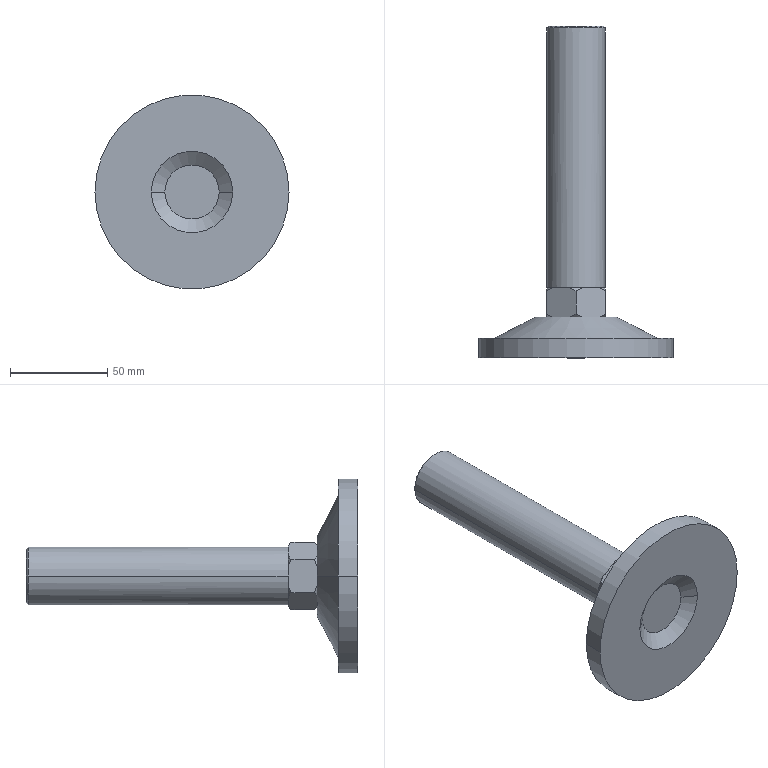Part | SolidWorks | features ICE 3, Chamfer 1, RevCut 1, Revolution 1 | 1 solid | 39 faces | box 100 x 171 x 100 mm | volume 216271 mm3 | cone 18 | plane 17 | cylinder 4 | commonest cylinder face diameters 30 x2 100 x2
STEP:
#1=CARTESIAN_POINT('',(14.,15.,0.));
#2=VERTEX_POINT('',#1);
#3=CARTESIAN_POINT('',(-14.,15.,0.));
#4=VERTEX_POINT('',#3);
#5=CARTESIAN_POINT('',(0.,15.,0.));
#6=DIRECTION('',(0.,1.,0.));
#7=DIRECTION('',(-1.,0.,0.));
#8=AXIS2_PLACEMENT_3D('',#5,#6,#7);
#9=CIRCLE('',#8,14.);
#10=EDGE_CURVE('',#2,#4,#9,.T.);
#11=ORIENTED_EDGE('',*,*,#10,.T.);
#12=CARTESIAN_POINT('',(-21.,10.,0.));
#13=VERTEX_POINT('',#12);
#14=CARTESIAN_POINT('',(-14.,15.,0.));
#15=DIRECTION('',(-0.8137,-0.5812,0.));
#16=VECTOR('',#15,1000.);
#17=LINE('',#14,#16);
#18=EDGE_CURVE('',#4,#13,#17,.T.);
#19=ORIENTED_EDGE('',*,*,#18,.T.);
#20=CARTESIAN_POINT('',(21.,10.,0.));
#21=VERTEX_POINT('',#20);
#22=CARTESIAN_POINT('',(0.,10.,0.));
#23=DIRECTION('',(0.,-1.,0.));
#24=DIRECTION('',(-1.,0.,0.));
#25=AXIS2_PLACEMENT_3D('',#22,#23,#24);
#26=CIRCLE('',#25,21.);
#27=EDGE_CURVE('',#13,#21,#26,.T.);
#28=ORIENTED_EDGE('',*,*,#27,.T.);
#29=CARTESIAN_POINT('',(14.,15.,0.));
#30=DIRECTION('',(0.8137,-0.5812,0.));
#31=VECTOR('',#30,1000.);
#32=LINE('',#29,#31);
#33=EDGE_CURVE('',#2,#21,#32,.T.);
#34=ORIENTED_EDGE('',*,*,#33,.F.);
#35=EDGE_LOOP('',(#11,#19,#28,#34));
#36=FACE_OUTER_BOUND('',#35,.T.);
#37=CARTESIAN_POINT('',(0.,15.,0.));
#38=DIRECTION('',(0.,-1.,0.));
#39=DIRECTION('',(1.,0.,0.));
#40=AXIS2_PLACEMENT_3D('',#37,#38,#39);
#41=CONICAL_SURFACE('',#40,14.,0.9505);
#42=ADVANCED_FACE('',(#36),#41,.F.);
#43=CARTESIAN_POINT('',(50.,10.,0.));
#44=VERTEX_POINT('',#43);
#45=CARTESIAN_POINT('',(-50.,10.,0.));
#46=VERTEX_POINT('',#45);
#47=CARTESIAN_POINT('',(0.,10.,0.));
#48=DIRECTION('',(0.,-1.,0.));
#49=DIRECTION('',(-1.,0.,0.));
#50=AXIS2_PLACEMENT_3D('',#47,#48,#49);
#51=CIRCLE('',#50,50.);
#52=EDGE_CURVE('',#44,#46,#51,.T.);
#53=ORIENTED_EDGE('',*,*,#52,.F.);
#54=CARTESIAN_POINT('',(50.,20.,0.));
#55=VERTEX_POINT('',#54);
#56=CARTESIAN_POINT('',(50.,0.,0.));
#57=DIRECTION('',(0.,1.,0.));
#58=VECTOR('',#57,1000.);
#59=LINE('',#56,#58);
#60=EDGE_CURVE('',#44,#55,#59,.T.);
#61=ORIENTED_EDGE('',*,*,#60,.T.);
#62=CARTESIAN_POINT('',(-50.,20.,0.));
#63=VERTEX_POINT('',#62);
#64=CARTESIAN_POINT('',(0.,20.,0.));
#65=DIRECTION('',(0.,1.,0.));
#66=DIRECTION('',(-1.,0.,0.));
#67=AXIS2_PLACEMENT_3D('',#64,#65,#66);
#68=CIRCLE('',#67,50.);
#69=EDGE_CURVE('',#63,#55,#68,.T.);
#70=ORIENTED_EDGE('',*,*,#69,.F.);
#71=CARTESIAN_POINT('',(-50.,0.,0.));
#72=DIRECTION('',(0.,1.,0.));
#73=VECTOR('',#72,1000.);
#74=LINE('',#71,#73);
#75=EDGE_CURVE('',#46,#63,#74,.T.);
#76=ORIENTED_EDGE('',*,*,#75,.F.);
#77=EDGE_LOOP('',(#53,#61,#70,#76));
#78=FACE_OUTER_BOUND('',#77,.T.);
#79=CARTESIAN_POINT('',(0.,0.,0.));
#80=DIRECTION('',(0.,1.,0.));
#81=DIRECTION('',(-1.,0.,0.));
#82=AXIS2_PLACEMENT_3D('',#79,#80,#81);
#83=CYLINDRICAL_SURFACE('',#82,50.);
#84=ADVANCED_FACE('',(#78),#83,.T.);
#85=CARTESIAN_POINT('',(-14.,181.,0.));
#86=VERTEX_POINT('',#85);
#87=CARTESIAN_POINT('',(14.,181.,0.));
#88=VERTEX_POINT('',#87);
#89=CARTESIAN_POINT('',(0.,181.,0.));
#90=DIRECTION('',(0.,1.,0.));
#91=DIRECTION('',(1.,0.,0.));
#92=AXIS2_PLACEMENT_3D('',#89,#90,#91);
#93=CIRCLE('',#92,14.);
#94=EDGE_CURVE('',#86,#88,#93,.T.);
#95=ORIENTED_EDGE('',*,*,#94,.F.);
#96=CARTESIAN_POINT('',(-15.,180.,0.));
#97=VERTEX_POINT('',#96);
#98=CARTESIAN_POINT('',(-14.,181.,0.));
#99=DIRECTION('',(-0.7071,-0.7071,0.));
#100=VECTOR('',#99,1000.);
#101=LINE('',#98,#100);
#102=EDGE_CURVE('',#86,#97,#101,.T.);
#103=ORIENTED_EDGE('',*,*,#102,.T.);
#104=CARTESIAN_POINT('',(15.,180.,0.));
#105=VERTEX_POINT('',#104);
#106=CARTESIAN_POINT('',(0.,180.,0.));
#107=DIRECTION('',(0.,-1.,0.));
#108=DIRECTION('',(1.,0.,0.));
#109=AXIS2_PLACEMENT_3D('',#106,#107,#108);
#110=CIRCLE('',#109,15.);
#111=EDGE_CURVE('',#105,#97,#110,.T.);
#112=ORIENTED_EDGE('',*,*,#111,.F.);
#113=CARTESIAN_POINT('',(14.,181.,0.));
#114=DIRECTION('',(0.7071,-0.7071,0.));
#115=VECTOR('',#114,1000.);
#116=LINE('',#113,#115);
#117=EDGE_CURVE('',#88,#105,#116,.T.);
#118=ORIENTED_EDGE('',*,*,#117,.F.);
#119=EDGE_LOOP('',(#95,#103,#112,#118));
#120=FACE_OUTER_BOUND('',#119,.T.);
#121=CARTESIAN_POINT('',(0.,181.,0.));
#122=DIRECTION('',(0.,-1.,0.));
#123=DIRECTION('',(1.,0.,0.));
#124=AXIS2_PLACEMENT_3D('',#121,#122,#123);
#125=CONICAL_SURFACE('',#124,14.,0.7854);
#126=ADVANCED_FACE('',(#120),#125,.T.);
#127=CARTESIAN_POINT('',(7.5,46.,12.99));
#128=VERTEX_POINT('',#127);
#129=CARTESIAN_POINT('',(15.,46.,0.));
#130=VERTEX_POINT('',#129);
#131=CARTESIAN_POINT('',(0.,46.,0.));
#132=DIRECTION('',(0.,1.,0.));
#133=DIRECTION('',(0.,0.,1.));
#134=AXIS2_PLACEMENT_3D('',#131,#132,#133);
#135=CIRCLE('',#134,15.);
#136=EDGE_CURVE('',#128,#130,#135,.T.);
#137=ORIENTED_EDGE('',*,*,#136,.T.);
#138=CARTESIAN_POINT('',(15.,181.,0.));
#139=DIRECTION('',(0.,1.,0.));
#140=VECTOR('',#139,1000.);
#141=LINE('',#138,#140);
#142=EDGE_CURVE('',#130,#105,#141,.T.);
#143=ORIENTED_EDGE('',*,*,#142,.T.);
#144=ORIENTED_EDGE('',*,*,#111,.T.);
#145=CARTESIAN_POINT('',(-15.,46.,0.));
#146=VERTEX_POINT('',#145);
#147=CARTESIAN_POINT('',(-15.,181.,0.));
#148=DIRECTION('',(0.,1.,0.));
#149=VECTOR('',#148,1000.);
#150=LINE('',#147,#149);
#151=EDGE_CURVE('',#146,#97,#150,.T.);
#152=ORIENTED_EDGE('',*,*,#151,.F.);
#153=CARTESIAN_POINT('',(-7.5,46.,12.99));
#154=VERTEX_POINT('',#153);
#155=CARTESIAN_POINT('',(0.,46.,0.));
#156=DIRECTION('',(0.,1.,0.));
#157=DIRECTION('',(0.,0.,1.));
#158=AXIS2_PLACEMENT_3D('',#155,#156,#157);
#159=CIRCLE('',#158,15.);
#160=EDGE_CURVE('',#146,#154,#159,.T.);
#161=ORIENTED_EDGE('',*,*,#160,.T.);
#162=CARTESIAN_POINT('',(0.,46.,0.));
#163=DIRECTION('',(0.,1.,0.));
#164=DIRECTION('',(0.,0.,1.));
#165=AXIS2_PLACEMENT_3D('',#162,#163,#164);
#166=CIRCLE('',#165,15.);
#167=EDGE_CURVE('',#154,#128,#166,.T.);
#168=ORIENTED_EDGE('',*,*,#167,.T.);
#169=EDGE_LOOP('',(#137,#143,#144,#152,#161,#168));
#170=FACE_OUTER_BOUND('',#169,.T.);
#171=CARTESIAN_POINT('',(0.,181.,0.));
#172=DIRECTION('',(0.,1.,0.));
#173=DIRECTION('',(-1.,0.,0.));
#174=AXIS2_PLACEMENT_3D('',#171,#172,#173);
#175=CYLINDRICAL_SURFACE('',#174,15.);
#176=ADVANCED_FACE('',(#170),#175,.T.);
#177=CARTESIAN_POINT('',(-21.,31.,0.));
#178=VERTEX_POINT('',#177);
#179=CARTESIAN_POINT('',(21.,31.,0.));
#180=VERTEX_POINT('',#179);
#181=CARTESIAN_POINT('',(0.,31.,0.));
#182=DIRECTION('',(0.,1.,0.));
#183=DIRECTION('',(-1.,0.,0.));
#184=AXIS2_PLACEMENT_3D('',#181,#182,#183);
#185=CIRCLE('',#184,21.);
#186=EDGE_CURVE('',#178,#180,#185,.T.);
#187=ORIENTED_EDGE('',*,*,#186,.F.);
#188=CARTESIAN_POINT('',(-42.,20.,0.));
#189=VERTEX_POINT('',#188);
#190=CARTESIAN_POINT('',(-42.,20.,0.));
#191=DIRECTION('',(-0.8858,-0.464,0.));
#192=VECTOR('',#191,1000.);
#193=LINE('',#190,#192);
#194=EDGE_CURVE('',#178,#189,#193,.T.);
#195=ORIENTED_EDGE('',*,*,#194,.T.);
#196=CARTESIAN_POINT('',(42.,20.,0.));
#197=VERTEX_POINT('',#196);
#198=CARTESIAN_POINT('',(0.,20.,0.));
#199=DIRECTION('',(0.,1.,0.));
#200=DIRECTION('',(-1.,0.,0.));
#201=AXIS2_PLACEMENT_3D('',#198,#199,#200);
#202=CIRCLE('',#201,42.);
#203=EDGE_CURVE('',#189,#197,#202,.T.);
#204=ORIENTED_EDGE('',*,*,#203,.T.);
#205=CARTESIAN_POINT('',(42.,20.,0.));
#206=DIRECTION('',(0.8858,-0.464,0.));
#207=VECTOR('',#206,1000.);
#208=LINE('',#205,#207);
#209=EDGE_CURVE('',#180,#197,#208,.T.);
#210=ORIENTED_EDGE('',*,*,#209,.F.);
#211=EDGE_LOOP('',(#187,#195,#204,#210));
#212=FACE_OUTER_BOUND('',#211,.T.);
#213=CARTESIAN_POINT('',(0.,20.,0.));
#214=DIRECTION('',(0.,-1.,0.));
#215=DIRECTION('',(1.,0.,0.));
#216=AXIS2_PLACEMENT_3D('',#213,#214,#215);
#217=CONICAL_SURFACE('',#216,42.,1.088);
#218=ADVANCED_FACE('',(#212),#217,.T.);
#219=CARTESIAN_POINT('',(0.,20.,0.));
#220=DIRECTION('',(0.,1.,0.));
#221=DIRECTION('',(-1.,0.,0.));
#222=AXIS2_PLACEMENT_3D('',#219,#220,#221);
#223=CIRCLE('',#222,42.);
#224=EDGE_CURVE('',#197,#189,#223,.T.);
#225=ORIENTED_EDGE('',*,*,#224,.F.);
#226=ORIENTED_EDGE('',*,*,#203,.F.);
#227=EDGE_LOOP('',(#225,#226));
#228=FACE_BOUND('',#227,.T.);
#229=ORIENTED_EDGE('',*,*,#69,.T.);
#230=CARTESIAN_POINT('',(0.,20.,0.));
#231=DIRECTION('',(0.,1.,0.));
#232=DIRECTION('',(-1.,0.,0.));
#233=AXIS2_PLACEMENT_3D('',#230,#231,#232);
#234=CIRCLE('',#233,50.);
#235=EDGE_CURVE('',#55,#63,#234,.T.);
#236=ORIENTED_EDGE('',*,*,#235,.T.);
#237=EDGE_LOOP('',(#229,#236));
#238=FACE_OUTER_BOUND('',#237,.T.);
#239=CARTESIAN_POINT('',(60.,20.,0.));
#240=DIRECTION('',(0.,-1.,0.));
#241=DIRECTION('',(1.,0.,0.));
#242=AXIS2_PLACEMENT_3D('',#239,#240,#241);
#243=PLANE('',#242);
#244=ADVANCED_FACE('',(#228,#238),#243,.F.);
#245=CARTESIAN_POINT('',(15.,46.,5.029));
#246=VERTEX_POINT('',#245);
#247=CARTESIAN_POINT('',(11.855,46.,10.476));
#248=VERTEX_POINT('',#247);
#249=CARTESIAN_POINT('',(0.,46.,0.));
#250=DIRECTION('',(0.,-1.,0.));
#251=DIRECTION('',(1.,0.,0.));
#252=AXIS2_PLACEMENT_3D('',#249,#250,#251);
#253=CIRCLE('',#252,15.821);
#254=EDGE_CURVE('',#246,#248,#253,.T.);
#255=ORIENTED_EDGE('',*,*,#254,.F.);
#256=CARTESIAN_POINT('',(15.,46.,8.66));
#257=DIRECTION('',(0.,0.,-1.));
#258=VECTOR('',#257,1000.);
#259=LINE('',#256,#258);
#260=EDGE_CURVE('',#246,#130,#259,.T.);
#261=ORIENTED_EDGE('',*,*,#260,.T.);
#262=ORIENTED_EDGE('',*,*,#136,.F.);
#263=CARTESIAN_POINT('',(0.,46.,17.321));
#264=DIRECTION('',(0.866,0.,-0.5));
#265=VECTOR('',#264,1000.);
#266=LINE('',#263,#265);
#267=EDGE_CURVE('',#128,#248,#266,.T.);
#268=ORIENTED_EDGE('',*,*,#267,.T.);
#269=EDGE_LOOP('',(#255,#261,#262,#268));
#270=FACE_OUTER_BOUND('',#269,.T.);
#271=CARTESIAN_POINT('',(0.,46.,0.));
#272=DIRECTION('',(0.,1.,0.));
#273=DIRECTION('',(0.,0.,1.));
#274=AXIS2_PLACEMENT_3D('',#271,#272,#273);
#275=PLANE('',#274);
#276=ADVANCED_FACE('',(#270),#275,.T.);
#277=CARTESIAN_POINT('',(11.855,46.,-10.476));
#278=VERTEX_POINT('',#277);
#279=CARTESIAN_POINT('',(15.,46.,-5.029));
#280=VERTEX_POINT('',#279);
#281=CARTESIAN_POINT('',(0.,46.,0.));
#282=DIRECTION('',(0.,-1.,0.));
#283=DIRECTION('',(1.,0.,0.));
#284=AXIS2_PLACEMENT_3D('',#281,#282,#283);
#285=CIRCLE('',#284,15.821);
#286=EDGE_CURVE('',#278,#280,#285,.T.);
#287=ORIENTED_EDGE('',*,*,#286,.F.);
#288=CARTESIAN_POINT('',(7.5,46.,-12.99));
#289=VERTEX_POINT('',#288);
#290=CARTESIAN_POINT('',(15.,46.,-8.66));
#291=DIRECTION('',(-0.866,0.,-0.5));
#292=VECTOR('',#291,1000.);
#293=LINE('',#290,#292);
#294=EDGE_CURVE('',#278,#289,#293,.T.);
#295=ORIENTED_EDGE('',*,*,#294,.T.);
#296=CARTESIAN_POINT('',(0.,46.,0.));
#297=DIRECTION('',(0.,1.,0.));
#298=DIRECTION('',(0.,0.,1.));
#299=AXIS2_PLACEMENT_3D('',#296,#297,#298);
#300=CIRCLE('',#299,15.);
#301=EDGE_CURVE('',#130,#289,#300,.T.);
#302=ORIENTED_EDGE('',*,*,#301,.F.);
#303=CARTESIAN_POINT('',(15.,46.,8.66));
#304=DIRECTION('',(0.,0.,-1.));
#305=VECTOR('',#304,1000.);
#306=LINE('',#303,#305);
#307=EDGE_CURVE('',#130,#280,#306,.T.);
#308=ORIENTED_EDGE('',*,*,#307,.T.);
#309=EDGE_LOOP('',(#287,#295,#302,#308));
#310=FACE_OUTER_BOUND('',#309,.T.);
#311=CARTESIAN_POINT('',(0.,46.,0.));
#312=DIRECTION('',(0.,1.,0.));
#313=DIRECTION('',(0.,0.,1.));
#314=AXIS2_PLACEMENT_3D('',#311,#312,#313);
#315=PLANE('',#314);
#316=ADVANCED_FACE('',(#310),#315,.T.);
#317=CARTESIAN_POINT('',(-3.145,46.,-15.505));
#318=VERTEX_POINT('',#317);
#319=CARTESIAN_POINT('',(3.145,46.,-15.505));
#320=VERTEX_POINT('',#319);
#321=CARTESIAN_POINT('',(0.,46.,0.));
#322=DIRECTION('',(0.,-1.,0.));
#323=DIRECTION('',(1.,0.,0.));
#324=AXIS2_PLACEMENT_3D('',#321,#322,#323);
#325=CIRCLE('',#324,15.821);
#326=EDGE_CURVE('',#318,#320,#325,.T.);
#327=ORIENTED_EDGE('',*,*,#326,.F.);
#328=CARTESIAN_POINT('',(-7.5,46.,-12.99));
#329=VERTEX_POINT('',#328);
#330=CARTESIAN_POINT('',(0.,46.,-17.321));
#331=DIRECTION('',(-0.866,0.,0.5));
#332=VECTOR('',#331,1000.);
#333=LINE('',#330,#332);
#334=EDGE_CURVE('',#318,#329,#333,.T.);
#335=ORIENTED_EDGE('',*,*,#334,.T.);
#336=CARTESIAN_POINT('',(0.,46.,0.));
#337=DIRECTION('',(0.,1.,0.));
#338=DIRECTION('',(0.,0.,1.));
#339=AXIS2_PLACEMENT_3D('',#336,#337,#338);
#340=CIRCLE('',#339,15.);
#341=EDGE_CURVE('',#289,#329,#340,.T.);
#342=ORIENTED_EDGE('',*,*,#341,.F.);
#343=CARTESIAN_POINT('',(15.,46.,-8.66));
#344=DIRECTION('',(-0.866,0.,-0.5));
#345=VECTOR('',#344,1000.);
#346=LINE('',#343,#345);
#347=EDGE_CURVE('',#289,#320,#346,.T.);
#348=ORIENTED_EDGE('',*,*,#347,.T.);
#349=EDGE_LOOP('',(#327,#335,#342,#348));
#350=FACE_OUTER_BOUND('',#349,.T.);
#351=CARTESIAN_POINT('',(0.,46.,0.));
#352=DIRECTION('',(0.,1.,0.));
#353=DIRECTION('',(0.,0.,1.));
#354=AXIS2_PLACEMENT_3D('',#351,#352,#353);
#355=PLANE('',#354);
#356=ADVANCED_FACE('',(#350),#355,.T.);
#357=CARTESIAN_POINT('',(-15.,46.,-5.029));
#358=VERTEX_POINT('',#357);
#359=CARTESIAN_POINT('',(-11.855,46.,-10.476));
#360=VERTEX_POINT('',#359);
#361=CARTESIAN_POINT('',(0.,46.,0.));
#362=DIRECTION('',(0.,-1.,0.));
#363=DIRECTION('',(1.,0.,0.));
#364=AXIS2_PLACEMENT_3D('',#361,#362,#363);
#365=CIRCLE('',#364,15.821);
#366=EDGE_CURVE('',#358,#360,#365,.T.);
#367=ORIENTED_EDGE('',*,*,#366,.F.);
#368=CARTESIAN_POINT('',(-15.,46.,-8.66));
#369=DIRECTION('',(0.,0.,1.));
#370=VECTOR('',#369,1000.);
#371=LINE('',#368,#370);
#372=EDGE_CURVE('',#358,#146,#371,.T.);
#373=ORIENTED_EDGE('',*,*,#372,.T.);
#374=CARTESIAN_POINT('',(0.,46.,0.));
#375=DIRECTION('',(0.,1.,0.));
#376=DIRECTION('',(0.,0.,1.));
#377=AXIS2_PLACEMENT_3D('',#374,#375,#376);
#378=CIRCLE('',#377,15.);
#379=EDGE_CURVE('',#329,#146,#378,.T.);
#380=ORIENTED_EDGE('',*,*,#379,.F.);
#381=CARTESIAN_POINT('',(0.,46.,-17.321));
#382=DIRECTION('',(-0.866,0.,0.5));
#383=VECTOR('',#382,1000.);
#384=LINE('',#381,#383);
#385=EDGE_CURVE('',#329,#360,#384,.T.);
#386=ORIENTED_EDGE('',*,*,#385,.T.);
#387=EDGE_LOOP('',(#367,#373,#380,#386));
#388=FACE_OUTER_BOUND('',#387,.T.);
#389=CARTESIAN_POINT('',(0.,46.,0.));
#390=DIRECTION('',(0.,1.,0.));
#391=DIRECTION('',(0.,0.,1.));
#392=AXIS2_PLACEMENT_3D('',#389,#390,#391);
#393=PLANE('',#392);
#394=ADVANCED_FACE('',(#388),#393,.T.);
#395=CARTESIAN_POINT('',(-11.855,46.,10.476));
#396=VERTEX_POINT('',#395);
#397=CARTESIAN_POINT('',(-15.,46.,5.029));
#398=VERTEX_POINT('',#397);
#399=CARTESIAN_POINT('',(0.,46.,0.));
#400=DIRECTION('',(0.,-1.,0.));
#401=DIRECTION('',(1.,0.,0.));
#402=AXIS2_PLACEMENT_3D('',#399,#400,#401);
#403=CIRCLE('',#402,15.821);
#404=EDGE_CURVE('',#396,#398,#403,.T.);
#405=ORIENTED_EDGE('',*,*,#404,.F.);
#406=CARTESIAN_POINT('',(-15.,46.,8.66));
#407=DIRECTION('',(0.866,0.,0.5));
#408=VECTOR('',#407,1000.);
#409=LINE('',#406,#408);
#410=EDGE_CURVE('',#396,#154,#409,.T.);
#411=ORIENTED_EDGE('',*,*,#410,.T.);
#412=ORIENTED_EDGE('',*,*,#160,.F.);
#413=CARTESIAN_POINT('',(-15.,46.,-8.66));
#414=DIRECTION('',(0.,0.,1.));
#415=VECTOR('',#414,1000.);
#416=LINE('',#413,#415);
#417=EDGE_CURVE('',#146,#398,#416,.T.);
#418=ORIENTED_EDGE('',*,*,#417,.T.);
#419=EDGE_LOOP('',(#405,#411,#412,#418));
#420=FACE_OUTER_BOUND('',#419,.T.);
#421=CARTESIAN_POINT('',(0.,46.,0.));
#422=DIRECTION('',(0.,1.,0.));
#423=DIRECTION('',(0.,0.,1.));
#424=AXIS2_PLACEMENT_3D('',#421,#422,#423);
#425=PLANE('',#424);
#426=ADVANCED_FACE('',(#420),#425,.T.);
#427=CARTESIAN_POINT('',(3.145,46.,15.505));
#428=VERTEX_POINT('',#427);
#429=CARTESIAN_POINT('',(-3.145,46.,15.505));
#430=VERTEX_POINT('',#429);
#431=CARTESIAN_POINT('',(0.,46.,0.));
#432=DIRECTION('',(0.,-1.,0.));
#433=DIRECTION('',(0.,0.,1.));
#434=AXIS2_PLACEMENT_3D('',#431,#432,#433);
#435=CIRCLE('',#434,15.821);
#436=EDGE_CURVE('',#428,#430,#435,.T.);
#437=ORIENTED_EDGE('',*,*,#436,.F.);
#438=CARTESIAN_POINT('',(0.,46.,17.321));
#439=DIRECTION('',(0.866,0.,-0.5));
#440=VECTOR('',#439,1000.);
#441=LINE('',#438,#440);
#442=EDGE_CURVE('',#428,#128,#441,.T.);
#443=ORIENTED_EDGE('',*,*,#442,.T.);
#444=ORIENTED_EDGE('',*,*,#167,.F.);
#445=CARTESIAN_POINT('',(-15.,46.,8.66));
#446=DIRECTION('',(0.866,0.,0.5));
#447=VECTOR('',#446,1000.);
#448=LINE('',#445,#447);
#449=EDGE_CURVE('',#154,#430,#448,.T.);
#450=ORIENTED_EDGE('',*,*,#449,.T.);
#451=EDGE_LOOP('',(#437,#443,#444,#450));
#452=FACE_OUTER_BOUND('',#451,.T.);
#453=CARTESIAN_POINT('',(0.,46.,0.));
#454=DIRECTION('',(0.,1.,0.));
#455=DIRECTION('',(0.,0.,1.));
#456=AXIS2_PLACEMENT_3D('',#453,#454,#455);
#457=PLANE('',#456);
#458=ADVANCED_FACE('',(#452),#457,.T.);
#459=CARTESIAN_POINT('',(0.,31.,0.));
#460=DIRECTION('',(0.,1.,0.));
#461=DIRECTION('',(-1.,0.,0.));
#462=AXIS2_PLACEMENT_3D('',#459,#460,#461);
#463=CIRCLE('',#462,21.);
#464=EDGE_CURVE('',#180,#178,#463,.T.);
#465=ORIENTED_EDGE('',*,*,#464,.T.);
#466=ORIENTED_EDGE('',*,*,#186,.T.);
#467=EDGE_LOOP('',(#465,#466));
#468=FACE_OUTER_BOUND('',#467,.T.);
#469=CARTESIAN_POINT('',(11.855,31.,-10.476));
#470=VERTEX_POINT('',#469);
#471=CARTESIAN_POINT('',(15.,31.,-5.029));
#472=VERTEX_POINT('',#471);
#473=CARTESIAN_POINT('',(0.,31.,0.));
#474=DIRECTION('',(0.,-1.,0.));
#475=DIRECTION('',(1.,0.,0.));
#476=AXIS2_PLACEMENT_3D('',#473,#474,#475);
#477=CIRCLE('',#476,15.821);
#478=EDGE_CURVE('',#470,#472,#477,.T.);
#479=ORIENTED_EDGE('',*,*,#478,.T.);
#480=CARTESIAN_POINT('',(15.,31.,5.029));
#481=VERTEX_POINT('',#480);
#482=CARTESIAN_POINT('',(15.,31.,8.66));
#483=DIRECTION('',(0.,0.,-1.));
#484=VECTOR('',#483,1000.);
#485=LINE('',#482,#484);
#486=EDGE_CURVE('',#481,#472,#485,.T.);
#487=ORIENTED_EDGE('',*,*,#486,.F.);
#488=CARTESIAN_POINT('',(11.855,31.,10.476));
#489=VERTEX_POINT('',#488);
#490=CARTESIAN_POINT('',(0.,31.,0.));
#491=DIRECTION('',(0.,-1.,0.));
#492=DIRECTION('',(1.,0.,0.));
#493=AXIS2_PLACEMENT_3D('',#490,#491,#492);
#494=CIRCLE('',#493,15.821);
#495=EDGE_CURVE('',#481,#489,#494,.T.);
#496=ORIENTED_EDGE('',*,*,#495,.T.);
#497=CARTESIAN_POINT('',(3.145,31.,15.505));
#498=VERTEX_POINT('',#497);
#499=CARTESIAN_POINT('',(0.,31.,17.321));
#500=DIRECTION('',(0.866,0.,-0.5));
#501=VECTOR('',#500,1000.);
#502=LINE('',#499,#501);
#503=EDGE_CURVE('',#498,#489,#502,.T.);
#504=ORIENTED_EDGE('',*,*,#503,.F.);
#505=CARTESIAN_POINT('',(-3.145,31.,15.505));
#506=VERTEX_POINT('',#505);
#507=CARTESIAN_POINT('',(0.,31.,0.));
#508=DIRECTION('',(0.,-1.,0.));
#509=DIRECTION('',(1.,0.,0.));
#510=AXIS2_PLACEMENT_3D('',#507,#508,#509);
#511=CIRCLE('',#510,15.821);
#512=EDGE_CURVE('',#498,#506,#511,.T.);
#513=ORIENTED_EDGE('',*,*,#512,.T.);
#514=CARTESIAN_POINT('',(-11.855,31.,10.476));
#515=VERTEX_POINT('',#514);
#516=CARTESIAN_POINT('',(-15.,31.,8.66));
#517=DIRECTION('',(0.866,0.,0.5));
#518=VECTOR('',#517,1000.);
#519=LINE('',#516,#518);
#520=EDGE_CURVE('',#515,#506,#519,.T.);
#521=ORIENTED_EDGE('',*,*,#520,.F.);
#522=CARTESIAN_POINT('',(-15.,31.,5.029));
#523=VERTEX_POINT('',#522);
#524=CARTESIAN_POINT('',(0.,31.,0.));
#525=DIRECTION('',(0.,-1.,0.));
#526=DIRECTION('',(1.,0.,0.));
#527=AXIS2_PLACEMENT_3D('',#524,#525,#526);
#528=CIRCLE('',#527,15.821);
#529=EDGE_CURVE('',#515,#523,#528,.T.);
#530=ORIENTED_EDGE('',*,*,#529,.T.);
#531=CARTESIAN_POINT('',(-15.,31.,-5.029));
#532=VERTEX_POINT('',#531);
#533=CARTESIAN_POINT('',(-15.,31.,-8.66));
#534=DIRECTION('',(0.,0.,1.));
#535=VECTOR('',#534,1000.);
#536=LINE('',#533,#535);
#537=EDGE_CURVE('',#532,#523,#536,.T.);
#538=ORIENTED_EDGE('',*,*,#537,.F.);
#539=CARTESIAN_POINT('',(-11.855,31.,-10.476));
#540=VERTEX_POINT('',#539);
#541=CARTESIAN_POINT('',(0.,31.,0.));
#542=DIRECTION('',(0.,-1.,0.));
#543=DIRECTION('',(1.,0.,0.));
#544=AXIS2_PLACEMENT_3D('',#541,#542,#543);
#545=CIRCLE('',#544,15.821);
#546=EDGE_CURVE('',#532,#540,#545,.T.);
#547=ORIENTED_EDGE('',*,*,#546,.T.);
#548=CARTESIAN_POINT('',(-3.145,31.,-15.505));
#549=VERTEX_POINT('',#548);
#550=CARTESIAN_POINT('',(0.,31.,-17.321));
#551=DIRECTION('',(-0.866,0.,0.5));
#552=VECTOR('',#551,1000.);
#553=LINE('',#550,#552);
#554=EDGE_CURVE('',#549,#540,#553,.T.);
#555=ORIENTED_EDGE('',*,*,#554,.F.);
#556=CARTESIAN_POINT('',(3.145,31.,-15.505));
#557=VERTEX_POINT('',#556);
#558=CARTESIAN_POINT('',(0.,31.,0.));
#559=DIRECTION('',(0.,-1.,0.));
#560=DIRECTION('',(1.,0.,0.));
#561=AXIS2_PLACEMENT_3D('',#558,#559,#560);
#562=CIRCLE('',#561,15.821);
#563=EDGE_CURVE('',#549,#557,#562,.T.);
#564=ORIENTED_EDGE('',*,*,#563,.T.);
#565=CARTESIAN_POINT('',(15.,31.,-8.66));
#566=DIRECTION('',(-0.866,0.,-0.5));
#567=VECTOR('',#566,1000.);
#568=LINE('',#565,#567);
#569=EDGE_CURVE('',#470,#557,#568,.T.);
#570=ORIENTED_EDGE('',*,*,#569,.F.);
#571=EDGE_LOOP('',(#479,#487,#496,#504,#513,#521,#530,#538,#547,#555,#564,#570));
#572=FACE_BOUND('',#571,.T.);
#573=CARTESIAN_POINT('',(21.,31.,0.));
#574=DIRECTION('',(0.,-1.,0.));
#575=DIRECTION('',(1.,0.,0.));
#576=AXIS2_PLACEMENT_3D('',#573,#574,#575);
#577=PLANE('',#576);
#578=ADVANCED_FACE('',(#468,#572),#577,.F.);
#579=ORIENTED_EDGE('',*,*,#194,.F.);
#580=ORIENTED_EDGE('',*,*,#464,.F.);
#581=ORIENTED_EDGE('',*,*,#209,.T.);
#582=ORIENTED_EDGE('',*,*,#224,.T.);
#583=EDGE_LOOP('',(#579,#580,#581,#582));
#584=FACE_OUTER_BOUND('',#583,.T.);
#585=CARTESIAN_POINT('',(0.,20.,0.));
#586=DIRECTION('',(0.,-1.,0.));
#587=DIRECTION('',(1.,0.,0.));
#588=AXIS2_PLACEMENT_3D('',#585,#586,#587);
#589=CONICAL_SURFACE('',#588,42.,1.088);
#590=ADVANCED_FACE('',(#584),#589,.T.);
#591=CARTESIAN_POINT('',(15.,44.5,-8.66));
#592=VERTEX_POINT('',#591);
#593=CARTESIAN_POINT('',(15.,32.5,-8.66));
#594=VERTEX_POINT('',#593);
#595=CARTESIAN_POINT('',(15.,46.,-8.66));
#596=DIRECTION('',(0.,-1.,0.));
#597=VECTOR('',#596,1000.);
#598=LINE('',#595,#597);
#599=EDGE_CURVE('',#592,#594,#598,.T.);
#600=ORIENTED_EDGE('',*,*,#599,.F.);
#601=CARTESIAN_POINT('',(15.,44.5,-8.66));
#602=CARTESIAN_POINT('',(15.,44.793,-8.073));
#603=CARTESIAN_POINT('',(15.,45.071,-7.474));
#604=CARTESIAN_POINT('',(15.,45.575,-6.264));
#605=CARTESIAN_POINT('',(15.,45.802,-5.651));
#606=CARTESIAN_POINT('',(15.,46.,-5.029));
#607=B_SPLINE_CURVE_WITH_KNOTS('',3,(#601,#602,#603,#604,#605,#606),.UNSPECIFIED.,.F.,.F.,(4,2,4),(0.01254,0.01449,0.01645),.UNSPECIFIED.);
#608=EDGE_CURVE('',#592,#280,#607,.T.);
#609=ORIENTED_EDGE('',*,*,#608,.T.);
#610=ORIENTED_EDGE('',*,*,#307,.F.);
#611=ORIENTED_EDGE('',*,*,#260,.F.);
#612=CARTESIAN_POINT('',(15.,44.5,8.66));
#613=VERTEX_POINT('',#612);
#614=CARTESIAN_POINT('',(15.,46.,5.029));
#615=CARTESIAN_POINT('',(15.,45.601,6.285));
#616=CARTESIAN_POINT('',(15.,45.086,7.489));
#617=CARTESIAN_POINT('',(15.,44.5,8.66));
#618=B_SPLINE_CURVE_WITH_KNOTS('',3,(#614,#615,#616,#617),.UNSPECIFIED.,.F.,.F.,(4,4),(0.02665,0.03058),.UNSPECIFIED.);
#619=EDGE_CURVE('',#246,#613,#618,.T.);
#620=ORIENTED_EDGE('',*,*,#619,.T.);
#621=CARTESIAN_POINT('',(15.,32.5,8.66));
#622=VERTEX_POINT('',#621);
#623=CARTESIAN_POINT('',(15.,46.,8.66));
#624=DIRECTION('',(0.,-1.,0.));
#625=VECTOR('',#624,1000.);
#626=LINE('',#623,#625);
#627=EDGE_CURVE('',#613,#622,#626,.T.);
#628=ORIENTED_EDGE('',*,*,#627,.T.);
#629=CARTESIAN_POINT('',(15.,32.5,8.66));
#630=CARTESIAN_POINT('',(15.,32.207,8.073));
#631=CARTESIAN_POINT('',(15.,31.929,7.474));
#632=CARTESIAN_POINT('',(15.,31.425,6.264));
#633=CARTESIAN_POINT('',(15.,31.198,5.651));
#634=CARTESIAN_POINT('',(15.,31.,5.029));
#635=B_SPLINE_CURVE_WITH_KNOTS('',3,(#629,#630,#631,#632,#633,#634),.UNSPECIFIED.,.F.,.F.,(4,2,4),(0.01254,0.01449,0.01645),.UNSPECIFIED.);
#636=EDGE_CURVE('',#622,#481,#635,.T.);
#637=ORIENTED_EDGE('',*,*,#636,.T.);
#638=ORIENTED_EDGE('',*,*,#486,.T.);
#639=CARTESIAN_POINT('',(15.,31.,-5.029));
#640=CARTESIAN_POINT('',(15.,31.399,-6.285));
#641=CARTESIAN_POINT('',(15.,31.914,-7.489));
#642=CARTESIAN_POINT('',(15.,32.5,-8.66));
#643=B_SPLINE_CURVE_WITH_KNOTS('',3,(#639,#640,#641,#642),.UNSPECIFIED.,.F.,.F.,(4,4),(0.02665,0.03058),.UNSPECIFIED.);
#644=EDGE_CURVE('',#472,#594,#643,.T.);
#645=ORIENTED_EDGE('',*,*,#644,.T.);
#646=EDGE_LOOP('',(#600,#609,#610,#611,#620,#628,#637,#638,#645));
#647=FACE_OUTER_BOUND('',#646,.T.);
#648=CARTESIAN_POINT('',(15.,46.,8.66));
#649=DIRECTION('',(-1.,0.,0.));
#650=DIRECTION('',(0.,-1.,0.));
#651=AXIS2_PLACEMENT_3D('',#648,#649,#650);
#652=PLANE('',#651);
#653=ADVANCED_FACE('',(#647),#652,.F.);
#654=CARTESIAN_POINT('',(0.,44.5,-17.321));
#655=VERTEX_POINT('',#654);
#656=CARTESIAN_POINT('',(0.,32.5,-17.321));
#657=VERTEX_POINT('',#656);
#658=CARTESIAN_POINT('',(0.,46.,-17.321));
#659=DIRECTION('',(0.,-1.,0.));
#660=VECTOR('',#659,1000.);
#661=LINE('',#658,#660);
#662=EDGE_CURVE('',#655,#657,#661,.T.);
#663=ORIENTED_EDGE('',*,*,#662,.F.);
#664=CARTESIAN_POINT('',(0.,44.5,-17.321));
#665=CARTESIAN_POINT('',(1.016,45.087,-16.734));
#666=CARTESIAN_POINT('',(2.059,45.602,-16.132));
#667=CARTESIAN_POINT('',(3.145,46.,-15.505));
#668=B_SPLINE_CURVE_WITH_KNOTS('',3,(#664,#665,#666,#667),.UNSPECIFIED.,.F.,.F.,(4,4),(0.01461,0.01854),.UNSPECIFIED.);
#669=EDGE_CURVE('',#655,#320,#668,.T.);
#670=ORIENTED_EDGE('',*,*,#669,.T.);
#671=ORIENTED_EDGE('',*,*,#347,.F.);
#672=ORIENTED_EDGE('',*,*,#294,.F.);
#673=CARTESIAN_POINT('',(11.855,46.,-10.476));
#674=CARTESIAN_POINT('',(12.396,45.802,-10.164));
#675=CARTESIAN_POINT('',(12.932,45.571,-9.854));
#676=CARTESIAN_POINT('',(13.982,45.066,-9.248));
#677=CARTESIAN_POINT('',(14.496,44.791,-8.951));
#678=CARTESIAN_POINT('',(15.,44.5,-8.66));
#679=B_SPLINE_CURVE_WITH_KNOTS('',3,(#673,#674,#675,#676,#677,#678),.UNSPECIFIED.,.F.,.F.,(4,2,4),(0.02875,0.03071,0.03267),.UNSPECIFIED.);
#680=EDGE_CURVE('',#278,#592,#679,.T.);
#681=ORIENTED_EDGE('',*,*,#680,.T.);
#682=ORIENTED_EDGE('',*,*,#599,.T.);
#683=CARTESIAN_POINT('',(15.,32.5,-8.66));
#684=CARTESIAN_POINT('',(13.984,31.913,-9.247));
#685=CARTESIAN_POINT('',(12.941,31.398,-9.849));
#686=CARTESIAN_POINT('',(11.855,31.,-10.476));
#687=B_SPLINE_CURVE_WITH_KNOTS('',3,(#683,#684,#685,#686),.UNSPECIFIED.,.F.,.F.,(4,4),(0.01461,0.01854),.UNSPECIFIED.);
#688=EDGE_CURVE('',#594,#470,#687,.T.);
#689=ORIENTED_EDGE('',*,*,#688,.T.);
#690=ORIENTED_EDGE('',*,*,#569,.T.);
#691=CARTESIAN_POINT('',(3.145,31.,-15.505));
#692=CARTESIAN_POINT('',(2.604,31.198,-15.817));
#693=CARTESIAN_POINT('',(2.068,31.429,-16.127));
#694=CARTESIAN_POINT('',(1.018,31.934,-16.733));
#695=CARTESIAN_POINT('',(0.5043,32.209,-17.029));
#696=CARTESIAN_POINT('',(0.,32.5,-17.321));
#697=B_SPLINE_CURVE_WITH_KNOTS('',3,(#691,#692,#693,#694,#695,#696),.UNSPECIFIED.,.F.,.F.,(4,2,4),(0.02875,0.03071,0.03267),.UNSPECIFIED.);
#698=EDGE_CURVE('',#557,#657,#697,.T.);
#699=ORIENTED_EDGE('',*,*,#698,.T.);
#700=EDGE_LOOP('',(#663,#670,#671,#672,#681,#682,#689,#690,#699));
#701=FACE_OUTER_BOUND('',#700,.T.);
#702=CARTESIAN_POINT('',(15.,46.,-8.66));
#703=DIRECTION('',(-0.5,0.,0.866));
#704=DIRECTION('',(0.866,0.,0.5));
#705=AXIS2_PLACEMENT_3D('',#702,#703,#704);
#706=PLANE('',#705);
#707=ADVANCED_FACE('',(#701),#706,.F.);
#708=CARTESIAN_POINT('',(-15.,44.5,-8.66));
#709=VERTEX_POINT('',#708);
#710=CARTESIAN_POINT('',(-15.,32.5,-8.66));
#711=VERTEX_POINT('',#710);
#712=CARTESIAN_POINT('',(-15.,46.,-8.66));
#713=DIRECTION('',(0.,-1.,0.));
#714=VECTOR('',#713,1000.);
#715=LINE('',#712,#714);
#716=EDGE_CURVE('',#709,#711,#715,.T.);
#717=ORIENTED_EDGE('',*,*,#716,.F.);
#718=CARTESIAN_POINT('',(-15.,44.5,-8.66));
#719=CARTESIAN_POINT('',(-13.984,45.087,-9.247));
#720=CARTESIAN_POINT('',(-12.941,45.602,-9.849));
#721=CARTESIAN_POINT('',(-11.855,46.,-10.476));
#722=B_SPLINE_CURVE_WITH_KNOTS('',3,(#718,#719,#720,#721),.UNSPECIFIED.,.F.,.F.,(4,4),(0.01461,0.01854),.UNSPECIFIED.);
#723=EDGE_CURVE('',#709,#360,#722,.T.);
#724=ORIENTED_EDGE('',*,*,#723,.T.);
#725=ORIENTED_EDGE('',*,*,#385,.F.);
#726=ORIENTED_EDGE('',*,*,#334,.F.);
#727=CARTESIAN_POINT('',(-3.145,46.,-15.505));
#728=CARTESIAN_POINT('',(-2.604,45.802,-15.817));
#729=CARTESIAN_POINT('',(-2.068,45.571,-16.127));
#730=CARTESIAN_POINT('',(-1.018,45.066,-16.733));
#731=CARTESIAN_POINT('',(-0.5043,44.791,-17.029));
#732=CARTESIAN_POINT('',(0.,44.5,-17.321));
#733=B_SPLINE_CURVE_WITH_KNOTS('',3,(#727,#728,#729,#730,#731,#732),.UNSPECIFIED.,.F.,.F.,(4,2,4),(0.02875,0.03071,0.03267),.UNSPECIFIED.);
#734=EDGE_CURVE('',#318,#655,#733,.T.);
#735=ORIENTED_EDGE('',*,*,#734,.T.);
#736=ORIENTED_EDGE('',*,*,#662,.T.);
#737=CARTESIAN_POINT('',(0.,32.5,-17.321));
#738=CARTESIAN_POINT('',(-1.016,31.913,-16.734));
#739=CARTESIAN_POINT('',(-2.059,31.398,-16.132));
#740=CARTESIAN_POINT('',(-3.145,31.,-15.505));
#741=B_SPLINE_CURVE_WITH_KNOTS('',3,(#737,#738,#739,#740),.UNSPECIFIED.,.F.,.F.,(4,4),(0.01461,0.01854),.UNSPECIFIED.);
#742=EDGE_CURVE('',#657,#549,#741,.T.);
#743=ORIENTED_EDGE('',*,*,#742,.T.);
#744=ORIENTED_EDGE('',*,*,#554,.T.);
#745=CARTESIAN_POINT('',(-11.855,31.,-10.476));
#746=CARTESIAN_POINT('',(-12.396,31.198,-10.164));
#747=CARTESIAN_POINT('',(-12.932,31.429,-9.854));
#748=CARTESIAN_POINT('',(-13.982,31.934,-9.248));
#749=CARTESIAN_POINT('',(-14.496,32.209,-8.951));
#750=CARTESIAN_POINT('',(-15.,32.5,-8.66));
#751=B_SPLINE_CURVE_WITH_KNOTS('',3,(#745,#746,#747,#748,#749,#750),.UNSPECIFIED.,.F.,.F.,(4,2,4),(0.02875,0.03071,0.03267),.UNSPECIFIED.);
#752=EDGE_CURVE('',#540,#711,#751,.T.);
#753=ORIENTED_EDGE('',*,*,#752,.T.);
#754=EDGE_LOOP('',(#717,#724,#725,#726,#735,#736,#743,#744,#753));
#755=FACE_OUTER_BOUND('',#754,.T.);
#756=CARTESIAN_POINT('',(0.,46.,-17.321));
#757=DIRECTION('',(0.5,0.,0.866));
#758=DIRECTION('',(0.866,0.,-0.5));
#759=AXIS2_PLACEMENT_3D('',#756,#757,#758);
#760=PLANE('',#759);
#761=ADVANCED_FACE('',(#755),#760,.F.);
#762=CARTESIAN_POINT('',(-15.,44.5,8.66));
#763=VERTEX_POINT('',#762);
#764=CARTESIAN_POINT('',(-15.,32.5,8.66));
#765=VERTEX_POINT('',#764);
#766=CARTESIAN_POINT('',(-15.,46.,8.66));
#767=DIRECTION('',(0.,-1.,0.));
#768=VECTOR('',#767,1000.);
#769=LINE('',#766,#768);
#770=EDGE_CURVE('',#763,#765,#769,.T.);
#771=ORIENTED_EDGE('',*,*,#770,.F.);
#772=CARTESIAN_POINT('',(-15.,44.5,8.66));
#773=CARTESIAN_POINT('',(-15.,44.793,8.073));
#774=CARTESIAN_POINT('',(-15.,45.071,7.474));
#775=CARTESIAN_POINT('',(-15.,45.575,6.264));
#776=CARTESIAN_POINT('',(-15.,45.802,5.651));
#777=CARTESIAN_POINT('',(-15.,46.,5.029));
#778=B_SPLINE_CURVE_WITH_KNOTS('',3,(#772,#773,#774,#775,#776,#777),.UNSPECIFIED.,.F.,.F.,(4,2,4),(0.01254,0.01449,0.01645),.UNSPECIFIED.);
#779=EDGE_CURVE('',#763,#398,#778,.T.);
#780=ORIENTED_EDGE('',*,*,#779,.T.);
#781=ORIENTED_EDGE('',*,*,#417,.F.);
#782=ORIENTED_EDGE('',*,*,#372,.F.);
#783=CARTESIAN_POINT('',(-15.,46.,-5.029));
#784=CARTESIAN_POINT('',(-15.,45.601,-6.285));
#785=CARTESIAN_POINT('',(-15.,45.086,-7.489));
#786=CARTESIAN_POINT('',(-15.,44.5,-8.66));
#787=B_SPLINE_CURVE_WITH_KNOTS('',3,(#783,#784,#785,#786),.UNSPECIFIED.,.F.,.F.,(4,4),(0.02665,0.03058),.UNSPECIFIED.);
#788=EDGE_CURVE('',#358,#709,#787,.T.);
#789=ORIENTED_EDGE('',*,*,#788,.T.);
#790=ORIENTED_EDGE('',*,*,#716,.T.);
#791=CARTESIAN_POINT('',(-15.,32.5,-8.66));
#792=CARTESIAN_POINT('',(-15.,32.207,-8.073));
#793=CARTESIAN_POINT('',(-15.,31.929,-7.474));
#794=CARTESIAN_POINT('',(-15.,31.425,-6.264));
#795=CARTESIAN_POINT('',(-15.,31.198,-5.651));
#796=CARTESIAN_POINT('',(-15.,31.,-5.029));
#797=B_SPLINE_CURVE_WITH_KNOTS('',3,(#791,#792,#793,#794,#795,#796),.UNSPECIFIED.,.F.,.F.,(4,2,4),(0.01254,0.01449,0.01645),.UNSPECIFIED.);
#798=EDGE_CURVE('',#711,#532,#797,.T.);
#799=ORIENTED_EDGE('',*,*,#798,.T.);
#800=ORIENTED_EDGE('',*,*,#537,.T.);
#801=CARTESIAN_POINT('',(-15.,31.,5.029));
#802=CARTESIAN_POINT('',(-15.,31.399,6.285));
#803=CARTESIAN_POINT('',(-15.,31.914,7.489));
#804=CARTESIAN_POINT('',(-15.,32.5,8.66));
#805=B_SPLINE_CURVE_WITH_KNOTS('',3,(#801,#802,#803,#804),.UNSPECIFIED.,.F.,.F.,(4,4),(0.02665,0.03058),.UNSPECIFIED.);
#806=EDGE_CURVE('',#523,#765,#805,.T.);
#807=ORIENTED_EDGE('',*,*,#806,.T.);
#808=EDGE_LOOP('',(#771,#780,#781,#782,#789,#790,#799,#800,#807));
#809=FACE_OUTER_BOUND('',#808,.T.);
#810=CARTESIAN_POINT('',(-15.,46.,-8.66));
#811=DIRECTION('',(1.,0.,0.));
#812=DIRECTION('',(0.,1.,0.));
#813=AXIS2_PLACEMENT_3D('',#810,#811,#812);
#814=PLANE('',#813);
#815=ADVANCED_FACE('',(#809),#814,.F.);
#816=CARTESIAN_POINT('',(0.,44.5,17.321));
#817=VERTEX_POINT('',#816);
#818=CARTESIAN_POINT('',(0.,32.5,17.321));
#819=VERTEX_POINT('',#818);
#820=CARTESIAN_POINT('',(0.,46.,17.321));
#821=DIRECTION('',(0.,-1.,0.));
#822=VECTOR('',#821,1000.);
#823=LINE('',#820,#822);
#824=EDGE_CURVE('',#817,#819,#823,.T.);
#825=ORIENTED_EDGE('',*,*,#824,.F.);
#826=CARTESIAN_POINT('',(0.,44.5,17.321));
#827=CARTESIAN_POINT('',(-1.016,45.087,16.734));
#828=CARTESIAN_POINT('',(-2.059,45.602,16.132));
#829=CARTESIAN_POINT('',(-3.145,46.,15.505));
#830=B_SPLINE_CURVE_WITH_KNOTS('',3,(#826,#827,#828,#829),.UNSPECIFIED.,.F.,.F.,(4,4),(0.01461,0.01854),.UNSPECIFIED.);
#831=EDGE_CURVE('',#817,#430,#830,.T.);
#832=ORIENTED_EDGE('',*,*,#831,.T.);
#833=ORIENTED_EDGE('',*,*,#449,.F.);
#834=ORIENTED_EDGE('',*,*,#410,.F.);
#835=CARTESIAN_POINT('',(-11.855,46.,10.476));
#836=CARTESIAN_POINT('',(-12.396,45.802,10.164));
#837=CARTESIAN_POINT('',(-12.932,45.571,9.854));
#838=CARTESIAN_POINT('',(-13.982,45.066,9.248));
#839=CARTESIAN_POINT('',(-14.496,44.791,8.951));
#840=CARTESIAN_POINT('',(-15.,44.5,8.66));
#841=B_SPLINE_CURVE_WITH_KNOTS('',3,(#835,#836,#837,#838,#839,#840),.UNSPECIFIED.,.F.,.F.,(4,2,4),(0.02875,0.03071,0.03267),.UNSPECIFIED.);
#842=EDGE_CURVE('',#396,#763,#841,.T.);
#843=ORIENTED_EDGE('',*,*,#842,.T.);
#844=ORIENTED_EDGE('',*,*,#770,.T.);
#845=CARTESIAN_POINT('',(-15.,32.5,8.66));
#846=CARTESIAN_POINT('',(-13.984,31.913,9.247));
#847=CARTESIAN_POINT('',(-12.941,31.398,9.849));
#848=CARTESIAN_POINT('',(-11.855,31.,10.476));
#849=B_SPLINE_CURVE_WITH_KNOTS('',3,(#845,#846,#847,#848),.UNSPECIFIED.,.F.,.F.,(4,4),(0.01461,0.01854),.UNSPECIFIED.);
#850=EDGE_CURVE('',#765,#515,#849,.T.);
#851=ORIENTED_EDGE('',*,*,#850,.T.);
#852=ORIENTED_EDGE('',*,*,#520,.T.);
#853=CARTESIAN_POINT('',(-3.145,31.,15.505));
#854=CARTESIAN_POINT('',(-2.604,31.198,15.817));
#855=CARTESIAN_POINT('',(-2.068,31.429,16.127));
#856=CARTESIAN_POINT('',(-1.018,31.934,16.733));
#857=CARTESIAN_POINT('',(-0.5043,32.209,17.029));
#858=CARTESIAN_POINT('',(0.,32.5,17.321));
#859=B_SPLINE_CURVE_WITH_KNOTS('',3,(#853,#854,#855,#856,#857,#858),.UNSPECIFIED.,.F.,.F.,(4,2,4),(0.02875,0.03071,0.03267),.UNSPECIFIED.);
#860=EDGE_CURVE('',#506,#819,#859,.T.);
#861=ORIENTED_EDGE('',*,*,#860,.T.);
#862=EDGE_LOOP('',(#825,#832,#833,#834,#843,#844,#851,#852,#861));
#863=FACE_OUTER_BOUND('',#862,.T.);
#864=CARTESIAN_POINT('',(-15.,46.,8.66));
#865=DIRECTION('',(0.5,0.,-0.866));
#866=DIRECTION('',(-0.866,0.,-0.5));
#867=AXIS2_PLACEMENT_3D('',#864,#865,#866);
#868=PLANE('',#867);
#869=ADVANCED_FACE('',(#863),#868,.F.);
#870=ORIENTED_EDGE('',*,*,#627,.F.);
#871=CARTESIAN_POINT('',(15.,44.5,8.66));
#872=CARTESIAN_POINT('',(13.984,45.087,9.247));
#873=CARTESIAN_POINT('',(12.941,45.602,9.849));
#874=CARTESIAN_POINT('',(11.855,46.,10.476));
#875=B_SPLINE_CURVE_WITH_KNOTS('',3,(#871,#872,#873,#874),.UNSPECIFIED.,.F.,.F.,(4,4),(0.01461,0.01854),.UNSPECIFIED.);
#876=EDGE_CURVE('',#613,#248,#875,.T.);
#877=ORIENTED_EDGE('',*,*,#876,.T.);
#878=ORIENTED_EDGE('',*,*,#267,.F.);
#879=ORIENTED_EDGE('',*,*,#442,.F.);
#880=CARTESIAN_POINT('',(3.145,46.,15.505));
#881=CARTESIAN_POINT('',(2.604,45.802,15.817));
#882=CARTESIAN_POINT('',(2.068,45.571,16.127));
#883=CARTESIAN_POINT('',(1.018,45.066,16.733));
#884=CARTESIAN_POINT('',(0.5043,44.791,17.029));
#885=CARTESIAN_POINT('',(0.,44.5,17.321));
#886=B_SPLINE_CURVE_WITH_KNOTS('',3,(#880,#881,#882,#883,#884,#885),.UNSPECIFIED.,.F.,.F.,(4,2,4),(0.02875,0.03071,0.03267),.UNSPECIFIED.);
#887=EDGE_CURVE('',#428,#817,#886,.T.);
#888=ORIENTED_EDGE('',*,*,#887,.T.);
#889=ORIENTED_EDGE('',*,*,#824,.T.);
#890=CARTESIAN_POINT('',(0.,32.5,17.321));
#891=CARTESIAN_POINT('',(1.016,31.913,16.734));
#892=CARTESIAN_POINT('',(2.059,31.398,16.132));
#893=CARTESIAN_POINT('',(3.145,31.,15.505));
#894=B_SPLINE_CURVE_WITH_KNOTS('',3,(#890,#891,#892,#893),.UNSPECIFIED.,.F.,.F.,(4,4),(0.01461,0.01854),.UNSPECIFIED.);
#895=EDGE_CURVE('',#819,#498,#894,.T.);
#896=ORIENTED_EDGE('',*,*,#895,.T.);
#897=ORIENTED_EDGE('',*,*,#503,.T.);
#898=CARTESIAN_POINT('',(11.855,31.,10.476));
#899=CARTESIAN_POINT('',(12.396,31.198,10.164));
#900=CARTESIAN_POINT('',(12.932,31.429,9.854));
#901=CARTESIAN_POINT('',(13.982,31.934,9.248));
#902=CARTESIAN_POINT('',(14.496,32.209,8.951));
#903=CARTESIAN_POINT('',(15.,32.5,8.66));
#904=B_SPLINE_CURVE_WITH_KNOTS('',3,(#898,#899,#900,#901,#902,#903),.UNSPECIFIED.,.F.,.F.,(4,2,4),(0.02875,0.03071,0.03267),.UNSPECIFIED.);
#905=EDGE_CURVE('',#489,#622,#904,.T.);
#906=ORIENTED_EDGE('',*,*,#905,.T.);
#907=EDGE_LOOP('',(#870,#877,#878,#879,#888,#889,#896,#897,#906));
#908=FACE_OUTER_BOUND('',#907,.T.);
#909=CARTESIAN_POINT('',(0.,46.,17.321));
#910=DIRECTION('',(-0.5,0.,-0.866));
#911=DIRECTION('',(-0.866,0.,0.5));
#912=AXIS2_PLACEMENT_3D('',#909,#910,#911);
#913=PLANE('',#912);
#914=ADVANCED_FACE('',(#908),#913,.F.);
#915=CARTESIAN_POINT('',(0.,181.,0.));
#916=DIRECTION('',(0.,1.,0.));
#917=DIRECTION('',(1.,0.,0.));
#918=AXIS2_PLACEMENT_3D('',#915,#916,#917);
#919=CIRCLE('',#918,14.);
#920=EDGE_CURVE('',#88,#86,#919,.T.);
#921=ORIENTED_EDGE('',*,*,#920,.T.);
#922=ORIENTED_EDGE('',*,*,#94,.T.);
#923=EDGE_LOOP('',(#921,#922));
#924=FACE_OUTER_BOUND('',#923,.T.);
#925=CARTESIAN_POINT('',(15.,181.,0.));
#926=DIRECTION('',(0.,-1.,0.));
#927=DIRECTION('',(1.,0.,0.));
#928=AXIS2_PLACEMENT_3D('',#925,#926,#927);
#929=PLANE('',#928);
#930=ADVANCED_FACE('',(#924),#929,.F.);
#931=ORIENTED_EDGE('',*,*,#142,.F.);
#932=ORIENTED_EDGE('',*,*,#301,.T.);
#933=ORIENTED_EDGE('',*,*,#341,.T.);
#934=ORIENTED_EDGE('',*,*,#379,.T.);
#935=ORIENTED_EDGE('',*,*,#151,.T.);
#936=CARTESIAN_POINT('',(0.,180.,0.));
#937=DIRECTION('',(0.,-1.,0.));
#938=DIRECTION('',(1.,0.,0.));
#939=AXIS2_PLACEMENT_3D('',#936,#937,#938);
#940=CIRCLE('',#939,15.);
#941=EDGE_CURVE('',#97,#105,#940,.T.);
#942=ORIENTED_EDGE('',*,*,#941,.T.);
#943=EDGE_LOOP('',(#931,#932,#933,#934,#935,#942));
#944=FACE_OUTER_BOUND('',#943,.T.);
#945=CARTESIAN_POINT('',(0.,181.,0.));
#946=DIRECTION('',(0.,1.,0.));
#947=DIRECTION('',(-1.,0.,0.));
#948=AXIS2_PLACEMENT_3D('',#945,#946,#947);
#949=CYLINDRICAL_SURFACE('',#948,15.);
#950=ADVANCED_FACE('',(#944),#949,.T.);
#951=ORIENTED_EDGE('',*,*,#905,.F.);
#952=ORIENTED_EDGE('',*,*,#495,.F.);
#953=ORIENTED_EDGE('',*,*,#636,.F.);
#954=EDGE_LOOP('',(#951,#952,#953));
#955=FACE_OUTER_BOUND('',#954,.T.);
#956=CARTESIAN_POINT('',(0.,32.5,0.));
#957=DIRECTION('',(0.,1.,0.));
#958=DIRECTION('',(-1.,0.,0.));
#959=AXIS2_PLACEMENT_3D('',#956,#957,#958);
#960=CONICAL_SURFACE('',#959,17.321,0.7854);
#961=ADVANCED_FACE('',(#955),#960,.T.);
#962=ORIENTED_EDGE('',*,*,#512,.F.);
#963=ORIENTED_EDGE('',*,*,#895,.F.);
#964=ORIENTED_EDGE('',*,*,#860,.F.);
#965=EDGE_LOOP('',(#962,#963,#964));
#966=FACE_OUTER_BOUND('',#965,.T.);
#967=CARTESIAN_POINT('',(0.,32.5,0.));
#968=DIRECTION('',(0.,1.,0.));
#969=DIRECTION('',(-1.,0.,0.));
#970=AXIS2_PLACEMENT_3D('',#967,#968,#969);
#971=CONICAL_SURFACE('',#970,17.321,0.7854);
#972=ADVANCED_FACE('',(#966),#971,.T.);
#973=ORIENTED_EDGE('',*,*,#529,.F.);
#974=ORIENTED_EDGE('',*,*,#850,.F.);
#975=ORIENTED_EDGE('',*,*,#806,.F.);
#976=EDGE_LOOP('',(#973,#974,#975));
#977=FACE_OUTER_BOUND('',#976,.T.);
#978=CARTESIAN_POINT('',(0.,32.5,0.));
#979=DIRECTION('',(0.,1.,0.));
#980=DIRECTION('',(-1.,0.,0.));
#981=AXIS2_PLACEMENT_3D('',#978,#979,#980);
#982=CONICAL_SURFACE('',#981,17.321,0.7854);
#983=ADVANCED_FACE('',(#977),#982,.T.);
#984=ORIENTED_EDGE('',*,*,#546,.F.);
#985=ORIENTED_EDGE('',*,*,#798,.F.);
#986=ORIENTED_EDGE('',*,*,#752,.F.);
#987=EDGE_LOOP('',(#984,#985,#986));
#988=FACE_OUTER_BOUND('',#987,.T.);
#989=CARTESIAN_POINT('',(0.,32.5,0.));
#990=DIRECTION('',(0.,1.,0.));
#991=DIRECTION('',(-1.,0.,0.));
#992=AXIS2_PLACEMENT_3D('',#989,#990,#991);
#993=CONICAL_SURFACE('',#992,17.321,0.7854);
#994=ADVANCED_FACE('',(#988),#993,.T.);
#995=ORIENTED_EDGE('',*,*,#563,.F.);
#996=ORIENTED_EDGE('',*,*,#742,.F.);
#997=ORIENTED_EDGE('',*,*,#698,.F.);
#998=EDGE_LOOP('',(#995,#996,#997));
#999=FACE_OUTER_BOUND('',#998,.T.);
#1000=CARTESIAN_POINT('',(0.,32.5,0.));
#1001=DIRECTION('',(0.,1.,0.));
#1002=DIRECTION('',(-1.,0.,0.));
#1003=AXIS2_PLACEMENT_3D('',#1000,#1001,#1002);
#1004=CONICAL_SURFACE('',#1003,17.321,0.7854);
#1005=ADVANCED_FACE('',(#999),#1004,.T.);
#1006=ORIENTED_EDGE('',*,*,#478,.F.);
#1007=ORIENTED_EDGE('',*,*,#688,.F.);
#1008=ORIENTED_EDGE('',*,*,#644,.F.);
#1009=EDGE_LOOP('',(#1006,#1007,#1008));
#1010=FACE_OUTER_BOUND('',#1009,.T.);
#1011=CARTESIAN_POINT('',(0.,32.5,0.));
#1012=DIRECTION('',(0.,1.,0.));
#1013=DIRECTION('',(-1.,0.,0.));
#1014=AXIS2_PLACEMENT_3D('',#1011,#1012,#1013);
#1015=CONICAL_SURFACE('',#1014,17.321,0.7854);
#1016=ADVANCED_FACE('',(#1010),#1015,.T.);
#1017=ORIENTED_EDGE('',*,*,#887,.F.);
#1018=ORIENTED_EDGE('',*,*,#436,.T.);
#1019=ORIENTED_EDGE('',*,*,#831,.F.);
#1020=EDGE_LOOP('',(#1017,#1018,#1019));
#1021=FACE_OUTER_BOUND('',#1020,.T.);
#1022=CARTESIAN_POINT('',(0.,46.,0.));
#1023=DIRECTION('',(0.,-1.,0.));
#1024=DIRECTION('',(1.,0.,0.));
#1025=AXIS2_PLACEMENT_3D('',#1022,#1023,#1024);
#1026=CONICAL_SURFACE('',#1025,15.821,0.7854);
#1027=ADVANCED_FACE('',(#1021),#1026,.T.);
#1028=ORIENTED_EDGE('',*,*,#842,.F.);
#1029=ORIENTED_EDGE('',*,*,#404,.T.);
#1030=ORIENTED_EDGE('',*,*,#779,.F.);
#1031=EDGE_LOOP('',(#1028,#1029,#1030));
#1032=FACE_OUTER_BOUND('',#1031,.T.);
#1033=CARTESIAN_POINT('',(0.,46.,0.));
#1034=DIRECTION('',(0.,-1.,0.));
#1035=DIRECTION('',(1.,0.,0.));
#1036=AXIS2_PLACEMENT_3D('',#1033,#1034,#1035);
#1037=CONICAL_SURFACE('',#1036,15.821,0.7854);
#1038=ADVANCED_FACE('',(#1032),#1037,.T.);
#1039=ORIENTED_EDGE('',*,*,#788,.F.);
#1040=ORIENTED_EDGE('',*,*,#366,.T.);
#1041=ORIENTED_EDGE('',*,*,#723,.F.);
#1042=EDGE_LOOP('',(#1039,#1040,#1041));
#1043=FACE_OUTER_BOUND('',#1042,.T.);
#1044=CARTESIAN_POINT('',(0.,46.,0.));
#1045=DIRECTION('',(0.,-1.,0.));
#1046=DIRECTION('',(1.,0.,0.));
#1047=AXIS2_PLACEMENT_3D('',#1044,#1045,#1046);
#1048=CONICAL_SURFACE('',#1047,15.821,0.7854);
#1049=ADVANCED_FACE('',(#1043),#1048,.T.);
#1050=ORIENTED_EDGE('',*,*,#734,.F.);
#1051=ORIENTED_EDGE('',*,*,#326,.T.);
#1052=ORIENTED_EDGE('',*,*,#669,.F.);
#1053=EDGE_LOOP('',(#1050,#1051,#1052));
#1054=FACE_OUTER_BOUND('',#1053,.T.);
#1055=CARTESIAN_POINT('',(0.,46.,0.));
#1056=DIRECTION('',(0.,-1.,0.));
#1057=DIRECTION('',(1.,0.,0.));
#1058=AXIS2_PLACEMENT_3D('',#1055,#1056,#1057);
#1059=CONICAL_SURFACE('',#1058,15.821,0.7854);
#1060=ADVANCED_FACE('',(#1054),#1059,.T.);
#1061=ORIENTED_EDGE('',*,*,#680,.F.);
#1062=ORIENTED_EDGE('',*,*,#286,.T.);
#1063=ORIENTED_EDGE('',*,*,#608,.F.);
#1064=EDGE_LOOP('',(#1061,#1062,#1063));
#1065=FACE_OUTER_BOUND('',#1064,.T.);
#1066=CARTESIAN_POINT('',(0.,46.,0.));
#1067=DIRECTION('',(0.,-1.,0.));
#1068=DIRECTION('',(1.,0.,0.));
#1069=AXIS2_PLACEMENT_3D('',#1066,#1067,#1068);
#1070=CONICAL_SURFACE('',#1069,15.821,0.7854);
#1071=ADVANCED_FACE('',(#1065),#1070,.T.);
#1072=ORIENTED_EDGE('',*,*,#254,.T.);
#1073=ORIENTED_EDGE('',*,*,#876,.F.);
#1074=ORIENTED_EDGE('',*,*,#619,.F.);
#1075=EDGE_LOOP('',(#1072,#1073,#1074));
#1076=FACE_OUTER_BOUND('',#1075,.T.);
#1077=CARTESIAN_POINT('',(0.,46.,0.));
#1078=DIRECTION('',(0.,-1.,0.));
#1079=DIRECTION('',(1.,0.,0.));
#1080=AXIS2_PLACEMENT_3D('',#1077,#1078,#1079);
#1081=CONICAL_SURFACE('',#1080,15.821,0.7854);
#1082=ADVANCED_FACE('',(#1076),#1081,.T.);
#1083=ORIENTED_EDGE('',*,*,#102,.F.);
#1084=ORIENTED_EDGE('',*,*,#920,.F.);
#1085=ORIENTED_EDGE('',*,*,#117,.T.);
#1086=ORIENTED_EDGE('',*,*,#941,.F.);
#1087=EDGE_LOOP('',(#1083,#1084,#1085,#1086));
#1088=FACE_OUTER_BOUND('',#1087,.T.);
#1089=CARTESIAN_POINT('',(0.,181.,0.));
#1090=DIRECTION('',(0.,-1.,0.));
#1091=DIRECTION('',(1.,0.,0.));
#1092=AXIS2_PLACEMENT_3D('',#1089,#1090,#1091);
#1093=CONICAL_SURFACE('',#1092,14.,0.7854);
#1094=ADVANCED_FACE('',(#1088),#1093,.T.);
#1095=ORIENTED_EDGE('',*,*,#60,.F.);
#1096=CARTESIAN_POINT('',(0.,10.,0.));
#1097=DIRECTION('',(0.,-1.,0.));
#1098=DIRECTION('',(-1.,0.,0.));
#1099=AXIS2_PLACEMENT_3D('',#1096,#1097,#1098);
#1100=CIRCLE('',#1099,50.);
#1101=EDGE_CURVE('',#46,#44,#1100,.T.);
#1102=ORIENTED_EDGE('',*,*,#1101,.F.);
#1103=ORIENTED_EDGE('',*,*,#75,.T.);
#1104=ORIENTED_EDGE('',*,*,#235,.F.);
#1105=EDGE_LOOP('',(#1095,#1102,#1103,#1104));
#1106=FACE_OUTER_BOUND('',#1105,.T.);
#1107=CARTESIAN_POINT('',(0.,0.,0.));
#1108=DIRECTION('',(0.,1.,0.));
#1109=DIRECTION('',(-1.,0.,0.));
#1110=AXIS2_PLACEMENT_3D('',#1107,#1108,#1109);
#1111=CYLINDRICAL_SURFACE('',#1110,50.);
#1112=ADVANCED_FACE('',(#1106),#1111,.T.);
#1113=ORIENTED_EDGE('',*,*,#1101,.T.);
#1114=ORIENTED_EDGE('',*,*,#52,.T.);
#1115=EDGE_LOOP('',(#1113,#1114));
#1116=FACE_OUTER_BOUND('',#1115,.T.);
#1117=CARTESIAN_POINT('',(0.,10.,0.));
#1118=DIRECTION('',(0.,-1.,0.));
#1119=DIRECTION('',(-1.,0.,0.));
#1120=AXIS2_PLACEMENT_3D('',#1117,#1118,#1119);
#1121=CIRCLE('',#1120,21.);
#1122=EDGE_CURVE('',#21,#13,#1121,.T.);
#1123=ORIENTED_EDGE('',*,*,#1122,.F.);
#1124=ORIENTED_EDGE('',*,*,#27,.F.);
#1125=EDGE_LOOP('',(#1123,#1124));
#1126=FACE_BOUND('',#1125,.T.);
#1127=CARTESIAN_POINT('',(-57.577,10.,-50.));
#1128=DIRECTION('',(0.,1.,0.));
#1129=DIRECTION('',(-1.,0.,0.));
#1130=AXIS2_PLACEMENT_3D('',#1127,#1128,#1129);
#1131=PLANE('',#1130);
#1132=ADVANCED_FACE('',(#1116,#1126),#1131,.F.);
#1133=ORIENTED_EDGE('',*,*,#10,.F.);
#1134=CARTESIAN_POINT('',(0.,15.,0.));
#1135=DIRECTION('',(0.,1.,0.));
#1136=DIRECTION('',(-1.,0.,0.));
#1137=AXIS2_PLACEMENT_3D('',#1134,#1135,#1136);
#1138=CIRCLE('',#1137,14.);
#1139=EDGE_CURVE('',#4,#2,#1138,.T.);
#1140=ORIENTED_EDGE('',*,*,#1139,.F.);
#1141=EDGE_LOOP('',(#1133,#1140));
#1142=FACE_OUTER_BOUND('',#1141,.T.);
#1143=CARTESIAN_POINT('',(0.,15.,0.));
#1144=DIRECTION('',(0.,1.,0.));
#1145=DIRECTION('',(-1.,0.,0.));
#1146=AXIS2_PLACEMENT_3D('',#1143,#1144,#1145);
#1147=PLANE('',#1146);
#1148=ADVANCED_FACE('',(#1142),#1147,.F.);
#1149=ORIENTED_EDGE('',*,*,#18,.F.);
#1150=ORIENTED_EDGE('',*,*,#1139,.T.);
#1151=ORIENTED_EDGE('',*,*,#33,.T.);
#1152=ORIENTED_EDGE('',*,*,#1122,.T.);
#1153=EDGE_LOOP('',(#1149,#1150,#1151,#1152));
#1154=FACE_OUTER_BOUND('',#1153,.T.);
#1155=CARTESIAN_POINT('',(0.,15.,0.));
#1156=DIRECTION('',(0.,-1.,0.));
#1157=DIRECTION('',(1.,0.,0.));
#1158=AXIS2_PLACEMENT_3D('',#1155,#1156,#1157);
#1159=CONICAL_SURFACE('',#1158,14.,0.9505);
#1160=ADVANCED_FACE('',(#1154),#1159,.F.);
#1161=CLOSED_SHELL('',(#42,#84,#126,#176,#218,#244,#276,#316,#356,#394,#426,#458,#578,#590,#653,#707,#761,#815,#869,#914,#930,#950,#961,#972,#983,#994,#1005,#1016,#1027,#1038,#1049,#1060,#1071,#1082,#1094,#1112,#1132,#1148,#1160));
#1162=MANIFOLD_SOLID_BREP('',#1161);
#1163=CARTESIAN_POINT('',(0.,0.,0.));
#1164=DIRECTION('',(0.,0.,1.));
#1165=DIRECTION('',(1.,0.,0.));
#1166=AXIS2_PLACEMENT_3D('',#1163,#1164,#1165);
#1167=(LENGTH_UNIT()NAMED_UNIT(*)SI_UNIT(.MILLI.,.METRE.));
#1168=UNCERTAINTY_MEASURE_WITH_UNIT(LENGTH_MEASURE(0.00001),#1167,'','');
#1169=(NAMED_UNIT(*)PLANE_ANGLE_UNIT()SI_UNIT($,.RADIAN.));
#1170=(NAMED_UNIT(*)SI_UNIT($,.STERADIAN.)SOLID_ANGLE_UNIT());
#1171=(GEOMETRIC_REPRESENTATION_CONTEXT(3)GLOBAL_UNCERTAINTY_ASSIGNED_CONTEXT((#1168))GLOBAL_UNIT_ASSIGNED_CONTEXT((#1167,#1169,#1170))REPRESENTATION_CONTEXT('',''));
#1172=ADVANCED_BREP_SHAPE_REPRESENTATION('',(#1162,#1166),#1171);